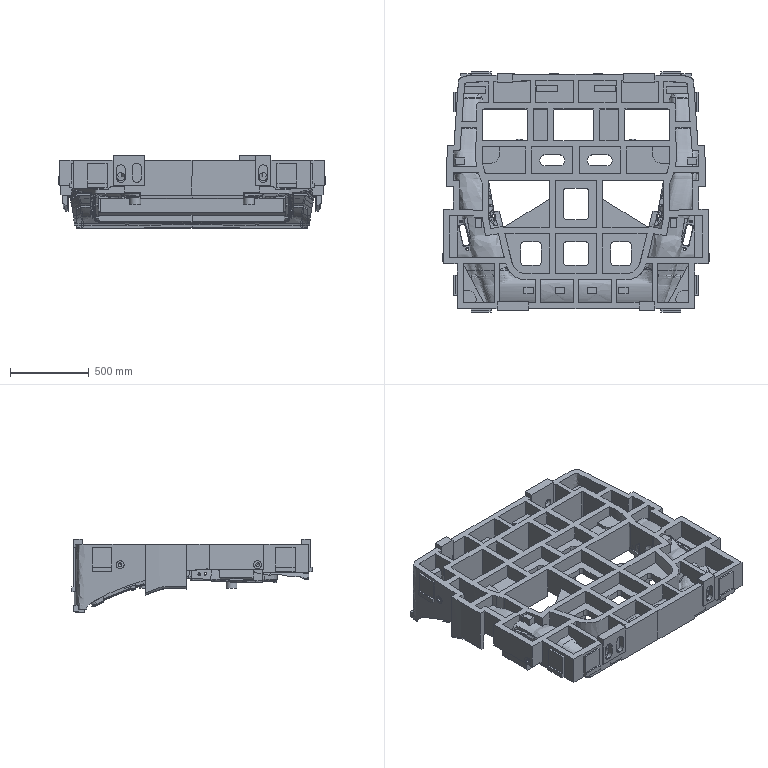Part | NX | features solid 2 | 6 solids | 2132 faces | box 1690 x 1520 x 462.798 mm | volume 242612279 mm3 | spline 1393 | plane 601 | cylinder 132 | cone 6 | commonest cylinder face diameters 52 x28 40 x18 2.1 x16 55 x10 20 x8 70 x8